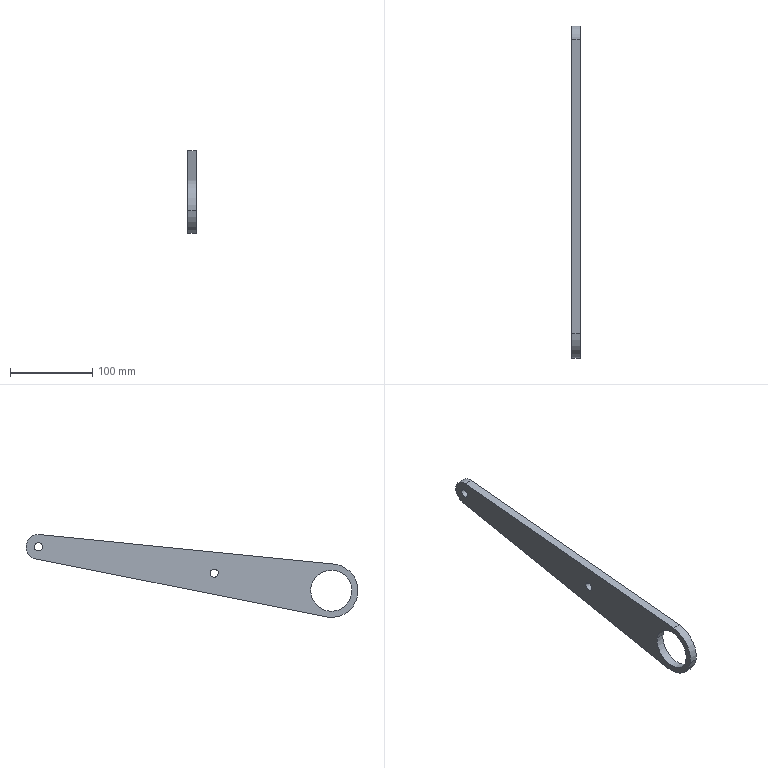Part | NX | features _-17232000 2 | 1 solid | 13 faces | box 10 x 403.429 x 100.813 mm | volume 170075 mm3 | cylinder 9 | plane 4 | commonest cylinder face diameters 10 x4 50 x2 65 x2 30 x1
STEP:
#1=CARTESIAN_POINT('',(-102.5,-285.524,-699.233));
#2=VERTEX_POINT('',#1);
#3=CARTESIAN_POINT('',(-102.5,-236.076,-691.826));
#4=VERTEX_POINT('',#3);
#5=CARTESIAN_POINT('',(-102.5,-260.8,-695.529));
#6=DIRECTION('',(1.,0.,0.));
#7=DIRECTION('',(0.,-0.989,-0.1481));
#8=AXIS2_PLACEMENT_3D('',#5,#6,#7);
#9=CIRCLE('',#8,25.);
#10=EDGE_CURVE('',#2,#4,#9,.T.);
#11=ORIENTED_EDGE('',*,*,#10,.F.);
#12=CARTESIAN_POINT('',(-92.5,-285.524,-699.233));
#13=VERTEX_POINT('',#12);
#14=CARTESIAN_POINT('',(-92.5,-285.524,-699.233));
#15=DIRECTION('',(-1.,0.,0.));
#16=VECTOR('',#15,1000.);
#17=LINE('',#14,#16);
#18=EDGE_CURVE('',#2,#13,#17,.F.);
#19=ORIENTED_EDGE('',*,*,#18,.T.);
#20=CARTESIAN_POINT('',(-92.5,-236.076,-691.826));
#21=VERTEX_POINT('',#20);
#22=CARTESIAN_POINT('',(-92.5,-260.8,-695.529));
#23=DIRECTION('',(-1.,0.,0.));
#24=DIRECTION('',(0.,0.989,0.1481));
#25=AXIS2_PLACEMENT_3D('',#22,#23,#24);
#26=CIRCLE('',#25,25.);
#27=EDGE_CURVE('',#21,#13,#26,.T.);
#28=ORIENTED_EDGE('',*,*,#27,.F.);
#29=CARTESIAN_POINT('',(-92.5,-236.076,-691.826));
#30=DIRECTION('',(-1.,0.,0.));
#31=VECTOR('',#30,1000.);
#32=LINE('',#29,#31);
#33=EDGE_CURVE('',#21,#4,#32,.T.);
#34=ORIENTED_EDGE('',*,*,#33,.T.);
#35=EDGE_LOOP('',(#11,#19,#28,#34));
#36=FACE_BOUND('',#35,.T.);
#37=CARTESIAN_POINT('',(-102.5,-260.8,-695.529));
#38=DIRECTION('',(1.,0.,0.));
#39=DIRECTION('',(0.,-0.989,-0.1481));
#40=AXIS2_PLACEMENT_3D('',#37,#38,#39);
#41=CYLINDRICAL_SURFACE('',#40,25.);
#42=ADVANCED_FACE('',(#36),#41,.F.);
#43=ORIENTED_EDGE('',*,*,#33,.F.);
#44=CARTESIAN_POINT('',(-92.5,-260.8,-695.529));
#45=DIRECTION('',(-1.,0.,0.));
#46=DIRECTION('',(0.,-0.989,-0.1481));
#47=AXIS2_PLACEMENT_3D('',#44,#45,#46);
#48=CIRCLE('',#47,25.);
#49=EDGE_CURVE('',#13,#21,#48,.T.);
#50=ORIENTED_EDGE('',*,*,#49,.F.);
#51=ORIENTED_EDGE('',*,*,#18,.F.);
#52=CARTESIAN_POINT('',(-102.5,-260.8,-695.529));
#53=DIRECTION('',(1.,0.,0.));
#54=DIRECTION('',(0.,0.989,0.1481));
#55=AXIS2_PLACEMENT_3D('',#52,#53,#54);
#56=CIRCLE('',#55,25.);
#57=EDGE_CURVE('',#4,#2,#56,.T.);
#58=ORIENTED_EDGE('',*,*,#57,.F.);
#59=EDGE_LOOP('',(#43,#50,#51,#58));
#60=FACE_BOUND('',#59,.T.);
#61=CARTESIAN_POINT('',(-102.5,-260.8,-695.529));
#62=DIRECTION('',(1.,0.,0.));
#63=DIRECTION('',(0.,-0.989,-0.1481));
#64=AXIS2_PLACEMENT_3D('',#61,#62,#63);
#65=CYLINDRICAL_SURFACE('',#64,25.);
#66=ADVANCED_FACE('',(#60),#65,.F.);
#67=CARTESIAN_POINT('',(-102.5,90.185,-642.957));
#68=VERTEX_POINT('',#67);
#69=CARTESIAN_POINT('',(-102.5,100.074,-641.476));
#70=VERTEX_POINT('',#69);
#71=CARTESIAN_POINT('',(-102.5,95.129,-642.216));
#72=DIRECTION('',(1.,0.,0.));
#73=DIRECTION('',(0.,-0.989,-0.1481));
#74=AXIS2_PLACEMENT_3D('',#71,#72,#73);
#75=CIRCLE('',#74,5.);
#76=EDGE_CURVE('',#68,#70,#75,.T.);
#77=ORIENTED_EDGE('',*,*,#76,.F.);
#78=CARTESIAN_POINT('',(-92.5,90.185,-642.957));
#79=VERTEX_POINT('',#78);
#80=CARTESIAN_POINT('',(-92.5,90.185,-642.957));
#81=DIRECTION('',(-1.,0.,0.));
#82=VECTOR('',#81,1000.);
#83=LINE('',#80,#82);
#84=EDGE_CURVE('',#79,#68,#83,.T.);
#85=ORIENTED_EDGE('',*,*,#84,.F.);
#86=CARTESIAN_POINT('',(-92.5,100.074,-641.476));
#87=VERTEX_POINT('',#86);
#88=CARTESIAN_POINT('',(-92.5,95.129,-642.216));
#89=DIRECTION('',(-1.,0.,0.));
#90=DIRECTION('',(0.,0.989,0.1481));
#91=AXIS2_PLACEMENT_3D('',#88,#89,#90);
#92=CIRCLE('',#91,5.);
#93=EDGE_CURVE('',#87,#79,#92,.T.);
#94=ORIENTED_EDGE('',*,*,#93,.F.);
#95=CARTESIAN_POINT('',(-92.5,100.074,-641.476));
#96=DIRECTION('',(-1.,0.,0.));
#97=VECTOR('',#96,1000.);
#98=LINE('',#95,#97);
#99=EDGE_CURVE('',#70,#87,#98,.F.);
#100=ORIENTED_EDGE('',*,*,#99,.F.);
#101=EDGE_LOOP('',(#77,#85,#94,#100));
#102=FACE_BOUND('',#101,.T.);
#103=CARTESIAN_POINT('',(-102.5,95.129,-642.216));
#104=DIRECTION('',(1.,0.,0.));
#105=DIRECTION('',(0.,-0.989,-0.1481));
#106=AXIS2_PLACEMENT_3D('',#103,#104,#105);
#107=CYLINDRICAL_SURFACE('',#106,5.);
#108=ADVANCED_FACE('',(#102),#107,.F.);
#109=ORIENTED_EDGE('',*,*,#99,.T.);
#110=CARTESIAN_POINT('',(-92.5,95.129,-642.216));
#111=DIRECTION('',(-1.,0.,0.));
#112=DIRECTION('',(0.,-0.989,-0.1481));
#113=AXIS2_PLACEMENT_3D('',#110,#111,#112);
#114=CIRCLE('',#113,5.);
#115=EDGE_CURVE('',#79,#87,#114,.T.);
#116=ORIENTED_EDGE('',*,*,#115,.F.);
#117=ORIENTED_EDGE('',*,*,#84,.T.);
#118=CARTESIAN_POINT('',(-102.5,95.129,-642.216));
#119=DIRECTION('',(1.,0.,0.));
#120=DIRECTION('',(0.,0.989,0.1481));
#121=AXIS2_PLACEMENT_3D('',#118,#119,#120);
#122=CIRCLE('',#121,5.);
#123=EDGE_CURVE('',#70,#68,#122,.T.);
#124=ORIENTED_EDGE('',*,*,#123,.F.);
#125=EDGE_LOOP('',(#109,#116,#117,#124));
#126=FACE_BOUND('',#125,.T.);
#127=CARTESIAN_POINT('',(-102.5,95.129,-642.216));
#128=DIRECTION('',(1.,0.,0.));
#129=DIRECTION('',(0.,-0.989,-0.1481));
#130=AXIS2_PLACEMENT_3D('',#127,#128,#129);
#131=CYLINDRICAL_SURFACE('',#130,5.);
#132=ADVANCED_FACE('',(#126),#131,.F.);
#133=CARTESIAN_POINT('',(-102.5,-254.429,-727.399));
#134=VERTEX_POINT('',#133);
#135=CARTESIAN_POINT('',(-92.5,-254.429,-727.399));
#136=VERTEX_POINT('',#135);
#137=CARTESIAN_POINT('',(-102.5,-254.429,-727.399));
#138=DIRECTION('',(1.,0.,0.));
#139=VECTOR('',#138,1000.);
#140=LINE('',#137,#139);
#141=EDGE_CURVE('',#134,#136,#140,.T.);
#142=ORIENTED_EDGE('',*,*,#141,.F.);
#143=CARTESIAN_POINT('',(-102.5,98.07,-656.925));
#144=VERTEX_POINT('',#143);
#145=CARTESIAN_POINT('',(-102.5,98.07,-656.925));
#146=DIRECTION('',(0.,-0.9806,-0.196));
#147=VECTOR('',#146,1000.);
#148=LINE('',#145,#147);
#149=EDGE_CURVE('',#144,#134,#148,.T.);
#150=ORIENTED_EDGE('',*,*,#149,.F.);
#151=CARTESIAN_POINT('',(-92.5,98.07,-656.925));
#152=VERTEX_POINT('',#151);
#153=CARTESIAN_POINT('',(-92.5,98.07,-656.925));
#154=DIRECTION('',(-1.,0.,0.));
#155=VECTOR('',#154,1000.);
#156=LINE('',#153,#155);
#157=EDGE_CURVE('',#152,#144,#156,.T.);
#158=ORIENTED_EDGE('',*,*,#157,.F.);
#159=CARTESIAN_POINT('',(-92.5,-254.429,-727.399));
#160=DIRECTION('',(0.,0.9806,0.196));
#161=VECTOR('',#160,1000.);
#162=LINE('',#159,#161);
#163=EDGE_CURVE('',#136,#152,#162,.T.);
#164=ORIENTED_EDGE('',*,*,#163,.F.);
#165=EDGE_LOOP('',(#142,#150,#158,#164));
#166=FACE_BOUND('',#165,.T.);
#167=CARTESIAN_POINT('',(-102.5,98.07,-656.925));
#168=DIRECTION('',(0.,-0.196,0.9806));
#169=DIRECTION('',(0.,0.9806,0.196));
#170=AXIS2_PLACEMENT_3D('',#167,#168,#169);
#171=PLANE('',#170);
#172=ADVANCED_FACE('',(#166),#171,.F.);
#173=ORIENTED_EDGE('',*,*,#157,.T.);
#174=CARTESIAN_POINT('',(-102.5,93.631,-627.291));
#175=VERTEX_POINT('',#174);
#176=CARTESIAN_POINT('',(-102.5,95.129,-642.216));
#177=DIRECTION('',(-1.,0.,0.));
#178=DIRECTION('',(0.,-0.09987,0.995));
#179=AXIS2_PLACEMENT_3D('',#176,#177,#178);
#180=CIRCLE('',#179,15.);
#181=EDGE_CURVE('',#175,#144,#180,.T.);
#182=ORIENTED_EDGE('',*,*,#181,.F.);
#183=CARTESIAN_POINT('',(-92.5,93.631,-627.291));
#184=VERTEX_POINT('',#183);
#185=CARTESIAN_POINT('',(-102.5,93.631,-627.291));
#186=DIRECTION('',(1.,0.,0.));
#187=VECTOR('',#186,1000.);
#188=LINE('',#185,#187);
#189=EDGE_CURVE('',#175,#184,#188,.T.);
#190=ORIENTED_EDGE('',*,*,#189,.T.);
#191=CARTESIAN_POINT('',(-92.5,95.129,-642.216));
#192=DIRECTION('',(1.,0.,0.));
#193=DIRECTION('',(0.,0.196,-0.9806));
#194=AXIS2_PLACEMENT_3D('',#191,#192,#193);
#195=CIRCLE('',#194,15.);
#196=EDGE_CURVE('',#152,#184,#195,.T.);
#197=ORIENTED_EDGE('',*,*,#196,.F.);
#198=EDGE_LOOP('',(#173,#182,#190,#197));
#199=FACE_BOUND('',#198,.T.);
#200=CARTESIAN_POINT('',(-102.5,95.129,-642.216));
#201=DIRECTION('',(1.,0.,0.));
#202=DIRECTION('',(0.,-0.989,-0.1481));
#203=AXIS2_PLACEMENT_3D('',#200,#201,#202);
#204=CYLINDRICAL_SURFACE('',#203,15.);
#205=ADVANCED_FACE('',(#199),#204,.T.);
#206=ORIENTED_EDGE('',*,*,#27,.T.);
#207=ORIENTED_EDGE('',*,*,#49,.T.);
#208=EDGE_LOOP('',(#206,#207));
#209=FACE_BOUND('',#208,.T.);
#210=CARTESIAN_POINT('',(-92.5,-113.543,-673.472));
#211=VERTEX_POINT('',#210);
#212=CARTESIAN_POINT('',(-92.5,-123.432,-674.954));
#213=VERTEX_POINT('',#212);
#214=CARTESIAN_POINT('',(-92.5,-118.488,-674.213));
#215=DIRECTION('',(-1.,0.,0.));
#216=DIRECTION('',(0.,0.989,0.1481));
#217=AXIS2_PLACEMENT_3D('',#214,#215,#216);
#218=CIRCLE('',#217,5.);
#219=EDGE_CURVE('',#211,#213,#218,.T.);
#220=ORIENTED_EDGE('',*,*,#219,.T.);
#221=CARTESIAN_POINT('',(-92.5,-118.488,-674.213));
#222=DIRECTION('',(-1.,0.,0.));
#223=DIRECTION('',(0.,-0.989,-0.1481));
#224=AXIS2_PLACEMENT_3D('',#221,#222,#223);
#225=CIRCLE('',#224,5.);
#226=EDGE_CURVE('',#213,#211,#225,.T.);
#227=ORIENTED_EDGE('',*,*,#226,.T.);
#228=EDGE_LOOP('',(#220,#227));
#229=FACE_BOUND('',#228,.T.);
#230=ORIENTED_EDGE('',*,*,#93,.T.);
#231=ORIENTED_EDGE('',*,*,#115,.T.);
#232=EDGE_LOOP('',(#230,#231));
#233=FACE_BOUND('',#232,.T.);
#234=ORIENTED_EDGE('',*,*,#163,.T.);
#235=ORIENTED_EDGE('',*,*,#196,.T.);
#236=CARTESIAN_POINT('',(-92.5,-264.046,-663.192));
#237=VERTEX_POINT('',#236);
#238=CARTESIAN_POINT('',(-92.5,93.631,-627.291));
#239=DIRECTION('',(0.,-0.995,-0.09987));
#240=VECTOR('',#239,1000.);
#241=LINE('',#238,#240);
#242=EDGE_CURVE('',#184,#237,#241,.T.);
#243=ORIENTED_EDGE('',*,*,#242,.T.);
#244=CARTESIAN_POINT('',(-92.5,-292.941,-700.344));
#245=VERTEX_POINT('',#244);
#246=CARTESIAN_POINT('',(-92.5,-260.8,-695.529));
#247=DIRECTION('',(1.,0.,0.));
#248=DIRECTION('',(0.,-0.09987,0.995));
#249=AXIS2_PLACEMENT_3D('',#246,#247,#248);
#250=CIRCLE('',#249,32.5);
#251=EDGE_CURVE('',#237,#245,#250,.T.);
#252=ORIENTED_EDGE('',*,*,#251,.T.);
#253=CARTESIAN_POINT('',(-92.5,-260.8,-695.529));
#254=DIRECTION('',(1.,0.,0.));
#255=DIRECTION('',(0.,-0.989,-0.1481));
#256=AXIS2_PLACEMENT_3D('',#253,#254,#255);
#257=CIRCLE('',#256,32.5);
#258=EDGE_CURVE('',#245,#136,#257,.T.);
#259=ORIENTED_EDGE('',*,*,#258,.T.);
#260=EDGE_LOOP('',(#234,#235,#243,#252,#259));
#261=FACE_BOUND('',#260,.T.);
#262=CARTESIAN_POINT('',(-92.5,-260.8,-695.529));
#263=DIRECTION('',(-1.,0.,0.));
#264=DIRECTION('',(0.,0.989,0.1481));
#265=AXIS2_PLACEMENT_3D('',#262,#263,#264);
#266=PLANE('',#265);
#267=ADVANCED_FACE('',(#209,#229,#233,#261),#266,.F.);
#268=ORIENTED_EDGE('',*,*,#189,.F.);
#269=CARTESIAN_POINT('',(-102.5,-264.046,-663.192));
#270=VERTEX_POINT('',#269);
#271=CARTESIAN_POINT('',(-102.5,-264.046,-663.192));
#272=DIRECTION('',(0.,0.995,0.09987));
#273=VECTOR('',#272,1000.);
#274=LINE('',#271,#273);
#275=EDGE_CURVE('',#270,#175,#274,.T.);
#276=ORIENTED_EDGE('',*,*,#275,.F.);
#277=CARTESIAN_POINT('',(-92.5,-264.046,-663.192));
#278=DIRECTION('',(-1.,0.,0.));
#279=VECTOR('',#278,1000.);
#280=LINE('',#277,#279);
#281=EDGE_CURVE('',#237,#270,#280,.T.);
#282=ORIENTED_EDGE('',*,*,#281,.F.);
#283=ORIENTED_EDGE('',*,*,#242,.F.);
#284=EDGE_LOOP('',(#268,#276,#282,#283));
#285=FACE_BOUND('',#284,.T.);
#286=CARTESIAN_POINT('',(-102.5,-264.046,-663.192));
#287=DIRECTION('',(0.,0.09987,-0.995));
#288=DIRECTION('',(0.,-0.995,-0.09987));
#289=AXIS2_PLACEMENT_3D('',#286,#287,#288);
#290=PLANE('',#289);
#291=ADVANCED_FACE('',(#285),#290,.F.);
#292=CARTESIAN_POINT('',(-102.5,-292.941,-700.344));
#293=VERTEX_POINT('',#292);
#294=CARTESIAN_POINT('',(-92.5,-292.941,-700.344));
#295=DIRECTION('',(-1.,0.,0.));
#296=VECTOR('',#295,1000.);
#297=LINE('',#294,#296);
#298=EDGE_CURVE('',#245,#293,#297,.T.);
#299=ORIENTED_EDGE('',*,*,#298,.F.);
#300=ORIENTED_EDGE('',*,*,#251,.F.);
#301=ORIENTED_EDGE('',*,*,#281,.T.);
#302=CARTESIAN_POINT('',(-102.5,-260.8,-695.529));
#303=DIRECTION('',(-1.,0.,0.));
#304=DIRECTION('',(0.,-0.989,-0.1481));
#305=AXIS2_PLACEMENT_3D('',#302,#303,#304);
#306=CIRCLE('',#305,32.5);
#307=EDGE_CURVE('',#293,#270,#306,.T.);
#308=ORIENTED_EDGE('',*,*,#307,.F.);
#309=EDGE_LOOP('',(#299,#300,#301,#308));
#310=FACE_BOUND('',#309,.T.);
#311=CARTESIAN_POINT('',(-102.5,-260.8,-695.529));
#312=DIRECTION('',(1.,0.,0.));
#313=DIRECTION('',(0.,-0.989,-0.1481));
#314=AXIS2_PLACEMENT_3D('',#311,#312,#313);
#315=CYLINDRICAL_SURFACE('',#314,32.5);
#316=ADVANCED_FACE('',(#310),#315,.T.);
#317=CARTESIAN_POINT('',(-102.5,-260.8,-695.529));
#318=DIRECTION('',(-1.,0.,0.));
#319=DIRECTION('',(0.,0.196,-0.9806));
#320=AXIS2_PLACEMENT_3D('',#317,#318,#319);
#321=CIRCLE('',#320,32.5);
#322=EDGE_CURVE('',#134,#293,#321,.T.);
#323=ORIENTED_EDGE('',*,*,#322,.F.);
#324=ORIENTED_EDGE('',*,*,#141,.T.);
#325=ORIENTED_EDGE('',*,*,#258,.F.);
#326=ORIENTED_EDGE('',*,*,#298,.T.);
#327=EDGE_LOOP('',(#323,#324,#325,#326));
#328=FACE_BOUND('',#327,.T.);
#329=CARTESIAN_POINT('',(-102.5,-260.8,-695.529));
#330=DIRECTION('',(1.,0.,0.));
#331=DIRECTION('',(0.,-0.989,-0.1481));
#332=AXIS2_PLACEMENT_3D('',#329,#330,#331);
#333=CYLINDRICAL_SURFACE('',#332,32.5);
#334=ADVANCED_FACE('',(#328),#333,.T.);
#335=ORIENTED_EDGE('',*,*,#10,.T.);
#336=ORIENTED_EDGE('',*,*,#57,.T.);
#337=EDGE_LOOP('',(#335,#336));
#338=FACE_BOUND('',#337,.T.);
#339=CARTESIAN_POINT('',(-102.5,-123.432,-674.954));
#340=VERTEX_POINT('',#339);
#341=CARTESIAN_POINT('',(-102.5,-113.543,-673.472));
#342=VERTEX_POINT('',#341);
#343=CARTESIAN_POINT('',(-102.5,-118.488,-674.213));
#344=DIRECTION('',(1.,0.,0.));
#345=DIRECTION('',(0.,-0.989,-0.1481));
#346=AXIS2_PLACEMENT_3D('',#343,#344,#345);
#347=CIRCLE('',#346,5.);
#348=EDGE_CURVE('',#340,#342,#347,.T.);
#349=ORIENTED_EDGE('',*,*,#348,.T.);
#350=CARTESIAN_POINT('',(-102.5,-118.488,-674.213));
#351=DIRECTION('',(1.,0.,0.));
#352=DIRECTION('',(0.,0.989,0.1481));
#353=AXIS2_PLACEMENT_3D('',#350,#351,#352);
#354=CIRCLE('',#353,5.);
#355=EDGE_CURVE('',#342,#340,#354,.T.);
#356=ORIENTED_EDGE('',*,*,#355,.T.);
#357=EDGE_LOOP('',(#349,#356));
#358=FACE_BOUND('',#357,.T.);
#359=ORIENTED_EDGE('',*,*,#76,.T.);
#360=ORIENTED_EDGE('',*,*,#123,.T.);
#361=EDGE_LOOP('',(#359,#360));
#362=FACE_BOUND('',#361,.T.);
#363=ORIENTED_EDGE('',*,*,#307,.T.);
#364=ORIENTED_EDGE('',*,*,#275,.T.);
#365=ORIENTED_EDGE('',*,*,#181,.T.);
#366=ORIENTED_EDGE('',*,*,#149,.T.);
#367=ORIENTED_EDGE('',*,*,#322,.T.);
#368=EDGE_LOOP('',(#363,#364,#365,#366,#367));
#369=FACE_BOUND('',#368,.T.);
#370=CARTESIAN_POINT('',(-102.5,-260.8,-695.529));
#371=DIRECTION('',(-1.,0.,0.));
#372=DIRECTION('',(0.,0.989,0.1481));
#373=AXIS2_PLACEMENT_3D('',#370,#371,#372);
#374=PLANE('',#373);
#375=ADVANCED_FACE('',(#338,#358,#362,#369),#374,.T.);
#376=CARTESIAN_POINT('',(-92.5,-113.543,-673.472));
#377=DIRECTION('',(-1.,0.,0.));
#378=VECTOR('',#377,1000.);
#379=LINE('',#376,#378);
#380=EDGE_CURVE('',#211,#342,#379,.T.);
#381=ORIENTED_EDGE('',*,*,#380,.F.);
#382=ORIENTED_EDGE('',*,*,#226,.F.);
#383=CARTESIAN_POINT('',(-92.5,-123.432,-674.954));
#384=DIRECTION('',(-1.,0.,0.));
#385=VECTOR('',#384,1000.);
#386=LINE('',#383,#385);
#387=EDGE_CURVE('',#340,#213,#386,.F.);
#388=ORIENTED_EDGE('',*,*,#387,.F.);
#389=ORIENTED_EDGE('',*,*,#355,.F.);
#390=EDGE_LOOP('',(#381,#382,#388,#389));
#391=FACE_BOUND('',#390,.T.);
#392=CARTESIAN_POINT('',(-102.5,-118.488,-674.213));
#393=DIRECTION('',(1.,0.,0.));
#394=DIRECTION('',(0.,-0.989,-0.1481));
#395=AXIS2_PLACEMENT_3D('',#392,#393,#394);
#396=CYLINDRICAL_SURFACE('',#395,5.);
#397=ADVANCED_FACE('',(#391),#396,.F.);
#398=ORIENTED_EDGE('',*,*,#348,.F.);
#399=ORIENTED_EDGE('',*,*,#387,.T.);
#400=ORIENTED_EDGE('',*,*,#219,.F.);
#401=ORIENTED_EDGE('',*,*,#380,.T.);
#402=EDGE_LOOP('',(#398,#399,#400,#401));
#403=FACE_BOUND('',#402,.T.);
#404=CARTESIAN_POINT('',(-102.5,-118.488,-674.213));
#405=DIRECTION('',(1.,0.,0.));
#406=DIRECTION('',(0.,-0.989,-0.1481));
#407=AXIS2_PLACEMENT_3D('',#404,#405,#406);
#408=CYLINDRICAL_SURFACE('',#407,5.);
#409=ADVANCED_FACE('',(#403),#408,.F.);
#410=CLOSED_SHELL('',(#42,#66,#108,#132,#172,#205,#267,#291,#316,#334,#375,#397,#409));
#411=MANIFOLD_SOLID_BREP('',#410);
#412=(LENGTH_UNIT()NAMED_UNIT(*)SI_UNIT(.MILLI.,.METRE.));
#413=UNCERTAINTY_MEASURE_WITH_UNIT(LENGTH_MEASURE(0.00001),#412,'','');
#414=(NAMED_UNIT(*)PLANE_ANGLE_UNIT()SI_UNIT($,.RADIAN.));
#415=(NAMED_UNIT(*)SI_UNIT($,.STERADIAN.)SOLID_ANGLE_UNIT());
#416=(GEOMETRIC_REPRESENTATION_CONTEXT(3)GLOBAL_UNCERTAINTY_ASSIGNED_CONTEXT((#413))GLOBAL_UNIT_ASSIGNED_CONTEXT((#412,#414,#415))REPRESENTATION_CONTEXT('',''));
#417=ADVANCED_BREP_SHAPE_REPRESENTATION('',(#411),#416);